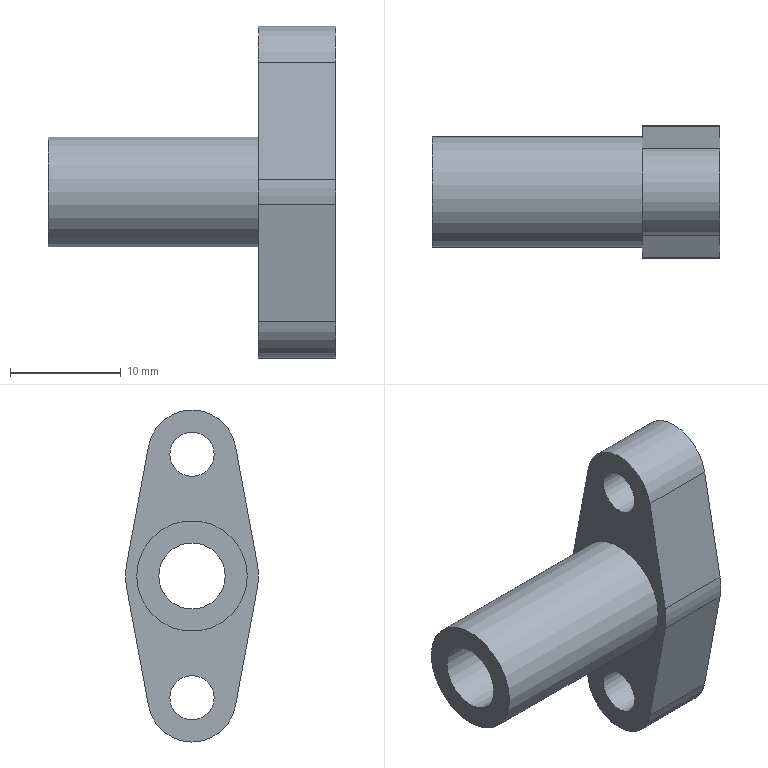Part | STEP file | 1-01.13 | 1 solid | 15 faces | box 26 x 12 x 30 mm | volume 2499 mm3 | cylinder 8 | plane 7 | commonest cylinder face diameters 4 x2 8 x2 12 x2 6 x1 10 x1
STEP:
#1=CARTESIAN_POINT('',(0.,0.,0.));
#2=DIRECTION('',(0.,0.,1.));
#3=DIRECTION('',(1.,0.,0.));
#4=AXIS2_PLACEMENT_3D('',#1,#2,#3);
#5=CARTESIAN_POINT('',(7.,5.9,-1.091));
#6=VERTEX_POINT('',#5);
#7=CARTESIAN_POINT('',(7.,5.9,1.091));
#8=VERTEX_POINT('',#7);
#9=CARTESIAN_POINT('',(7.,0.,0.));
#10=DIRECTION('',(1.,0.,0.));
#11=DIRECTION('',(0.,0.9833,-0.1818));
#12=AXIS2_PLACEMENT_3D('',#9,#10,#11);
#13=CIRCLE('',#12,6.);
#14=CARTESIAN_POINT('',(7.,8.898,0.));
#15=DIRECTION('',(1.,0.,0.));
#16=DIRECTION('',(0.,1.,0.));
#17=AXIS2_PLACEMENT_3D('',#14,#15,#16);
#18=PLANE('',#17);
#19=CARTESIAN_POINT('',(-8.898,0.));
#20=DIRECTION('',(0.9833,-0.1818));
#21=AXIS2_PLACEMENT_2D('',#19,#20);
#22=CIRCLE('',#21,6.);
#23=(GEOMETRIC_REPRESENTATION_CONTEXT(2)PARAMETRIC_REPRESENTATION_CONTEXT()REPRESENTATION_CONTEXT('',''));
#24=DEFINITIONAL_REPRESENTATION('',(#22),#23);
#25=PCURVE('',#18,#24);
#26=CARTESIAN_POINT('',(0.,0.,0.));
#27=DIRECTION('',(1.,0.,0.));
#28=DIRECTION('',(0.,0.9833,-0.1818));
#29=AXIS2_PLACEMENT_3D('',#26,#27,#28);
#30=CYLINDRICAL_SURFACE('',#29,6.);
#31=CARTESIAN_POINT('',(0.,7.));
#32=DIRECTION('',(1.,0.));
#33=VECTOR('',#32,1.);
#34=LINE('',#31,#33);
#35=(GEOMETRIC_REPRESENTATION_CONTEXT(2)PARAMETRIC_REPRESENTATION_CONTEXT()REPRESENTATION_CONTEXT('',''));
#36=DEFINITIONAL_REPRESENTATION('',(#34),#35);
#37=PCURVE('',#30,#36);
#38=SURFACE_CURVE('',#13,(#25,#37),.PCURVE_S1.);
#39=EDGE_CURVE('',#6,#8,#38,.T.);
#40=ORIENTED_EDGE('',*,*,#39,.T.);
#41=CARTESIAN_POINT('',(7.,3.933,11.727));
#42=VERTEX_POINT('',#41);
#43=CARTESIAN_POINT('',(7.,5.9,1.091));
#44=DIRECTION('',(0.,-0.1818,0.9833));
#45=VECTOR('',#44,1.);
#46=LINE('',#43,#45);
#47=CARTESIAN_POINT('',(-2.998,1.091));
#48=DIRECTION('',(-0.1818,0.9833));
#49=VECTOR('',#48,1.);
#50=LINE('',#47,#49);
#51=(GEOMETRIC_REPRESENTATION_CONTEXT(2)PARAMETRIC_REPRESENTATION_CONTEXT()REPRESENTATION_CONTEXT('',''));
#52=DEFINITIONAL_REPRESENTATION('',(#50),#51);
#53=PCURVE('',#18,#52);
#54=CARTESIAN_POINT('',(3.5,4.917,6.409));
#55=DIRECTION('',(0.,0.9833,0.1818));
#56=DIRECTION('',(0.,-0.1818,0.9833));
#57=AXIS2_PLACEMENT_3D('',#54,#55,#56);
#58=PLANE('',#57);
#59=CARTESIAN_POINT('',(-5.408,3.5));
#60=DIRECTION('',(1.,0.));
#61=VECTOR('',#60,1.);
#62=LINE('',#59,#61);
#63=(GEOMETRIC_REPRESENTATION_CONTEXT(2)PARAMETRIC_REPRESENTATION_CONTEXT()REPRESENTATION_CONTEXT('',''));
#64=DEFINITIONAL_REPRESENTATION('',(#62),#63);
#65=PCURVE('',#58,#64);
#66=SURFACE_CURVE('',#46,(#53,#65),.PCURVE_S1.);
#67=EDGE_CURVE('',#8,#42,#66,.T.);
#68=ORIENTED_EDGE('',*,*,#67,.T.);
#69=CARTESIAN_POINT('',(7.,-3.933,11.727));
#70=VERTEX_POINT('',#69);
#71=CARTESIAN_POINT('',(7.,0.,11.));
#72=DIRECTION('',(1.,0.,0.));
#73=DIRECTION('',(0.,0.9833,0.1818));
#74=AXIS2_PLACEMENT_3D('',#71,#72,#73);
#75=CIRCLE('',#74,4.);
#76=CARTESIAN_POINT('',(-8.898,11.));
#77=DIRECTION('',(0.9833,0.1818));
#78=AXIS2_PLACEMENT_2D('',#76,#77);
#79=CIRCLE('',#78,4.);
#80=(GEOMETRIC_REPRESENTATION_CONTEXT(2)PARAMETRIC_REPRESENTATION_CONTEXT()REPRESENTATION_CONTEXT('',''));
#81=DEFINITIONAL_REPRESENTATION('',(#79),#80);
#82=PCURVE('',#18,#81);
#83=CARTESIAN_POINT('',(0.,0.,11.));
#84=DIRECTION('',(1.,0.,0.));
#85=DIRECTION('',(0.,0.9833,0.1818));
#86=AXIS2_PLACEMENT_3D('',#83,#84,#85);
#87=CYLINDRICAL_SURFACE('',#86,4.);
#88=CARTESIAN_POINT('',(0.,7.));
#89=DIRECTION('',(1.,0.));
#90=VECTOR('',#89,1.);
#91=LINE('',#88,#90);
#92=(GEOMETRIC_REPRESENTATION_CONTEXT(2)PARAMETRIC_REPRESENTATION_CONTEXT()REPRESENTATION_CONTEXT('',''));
#93=DEFINITIONAL_REPRESENTATION('',(#91),#92);
#94=PCURVE('',#87,#93);
#95=SURFACE_CURVE('',#75,(#82,#94),.PCURVE_S1.);
#96=EDGE_CURVE('',#42,#70,#95,.T.);
#97=ORIENTED_EDGE('',*,*,#96,.T.);
#98=CARTESIAN_POINT('',(7.,-5.9,1.091));
#99=VERTEX_POINT('',#98);
#100=CARTESIAN_POINT('',(7.,-3.933,11.727));
#101=DIRECTION('',(0.,-0.1818,-0.9833));
#102=VECTOR('',#101,1.);
#103=LINE('',#100,#102);
#104=CARTESIAN_POINT('',(-12.832,11.727));
#105=DIRECTION('',(-0.1818,-0.9833));
#106=VECTOR('',#105,1.);
#107=LINE('',#104,#106);
#108=(GEOMETRIC_REPRESENTATION_CONTEXT(2)PARAMETRIC_REPRESENTATION_CONTEXT()REPRESENTATION_CONTEXT('',''));
#109=DEFINITIONAL_REPRESENTATION('',(#107),#108);
#110=PCURVE('',#18,#109);
#111=CARTESIAN_POINT('',(3.5,-4.917,6.409));
#112=DIRECTION('',(0.,-0.9833,0.1818));
#113=DIRECTION('',(0.,-0.1818,-0.9833));
#114=AXIS2_PLACEMENT_3D('',#111,#112,#113);
#115=PLANE('',#114);
#116=CARTESIAN_POINT('',(-5.408,3.5));
#117=DIRECTION('',(1.,0.));
#118=VECTOR('',#117,1.);
#119=LINE('',#116,#118);
#120=(GEOMETRIC_REPRESENTATION_CONTEXT(2)PARAMETRIC_REPRESENTATION_CONTEXT()REPRESENTATION_CONTEXT('',''));
#121=DEFINITIONAL_REPRESENTATION('',(#119),#120);
#122=PCURVE('',#115,#121);
#123=SURFACE_CURVE('',#103,(#110,#122),.PCURVE_S1.);
#124=EDGE_CURVE('',#70,#99,#123,.T.);
#125=ORIENTED_EDGE('',*,*,#124,.T.);
#126=CARTESIAN_POINT('',(7.,-5.9,-1.091));
#127=VERTEX_POINT('',#126);
#128=CARTESIAN_POINT('',(7.,0.,0.));
#129=DIRECTION('',(1.,0.,0.));
#130=DIRECTION('',(0.,-0.9833,0.1818));
#131=AXIS2_PLACEMENT_3D('',#128,#129,#130);
#132=CIRCLE('',#131,6.);
#133=CARTESIAN_POINT('',(-8.898,0.));
#134=DIRECTION('',(-0.9833,0.1818));
#135=AXIS2_PLACEMENT_2D('',#133,#134);
#136=CIRCLE('',#135,6.);
#137=(GEOMETRIC_REPRESENTATION_CONTEXT(2)PARAMETRIC_REPRESENTATION_CONTEXT()REPRESENTATION_CONTEXT('',''));
#138=DEFINITIONAL_REPRESENTATION('',(#136),#137);
#139=PCURVE('',#18,#138);
#140=CARTESIAN_POINT('',(0.,0.,0.));
#141=DIRECTION('',(1.,0.,0.));
#142=DIRECTION('',(0.,-0.9833,0.1818));
#143=AXIS2_PLACEMENT_3D('',#140,#141,#142);
#144=CYLINDRICAL_SURFACE('',#143,6.);
#145=CARTESIAN_POINT('',(0.,7.));
#146=DIRECTION('',(1.,0.));
#147=VECTOR('',#146,1.);
#148=LINE('',#145,#147);
#149=(GEOMETRIC_REPRESENTATION_CONTEXT(2)PARAMETRIC_REPRESENTATION_CONTEXT()REPRESENTATION_CONTEXT('',''));
#150=DEFINITIONAL_REPRESENTATION('',(#148),#149);
#151=PCURVE('',#144,#150);
#152=SURFACE_CURVE('',#132,(#139,#151),.PCURVE_S1.);
#153=EDGE_CURVE('',#99,#127,#152,.T.);
#154=ORIENTED_EDGE('',*,*,#153,.T.);
#155=CARTESIAN_POINT('',(7.,-3.933,-11.727));
#156=VERTEX_POINT('',#155);
#157=CARTESIAN_POINT('',(7.,-5.9,-1.091));
#158=DIRECTION('',(0.,0.1818,-0.9833));
#159=VECTOR('',#158,1.);
#160=LINE('',#157,#159);
#161=CARTESIAN_POINT('',(-14.798,-1.091));
#162=DIRECTION('',(0.1818,-0.9833));
#163=VECTOR('',#162,1.);
#164=LINE('',#161,#163);
#165=(GEOMETRIC_REPRESENTATION_CONTEXT(2)PARAMETRIC_REPRESENTATION_CONTEXT()REPRESENTATION_CONTEXT('',''));
#166=DEFINITIONAL_REPRESENTATION('',(#164),#165);
#167=PCURVE('',#18,#166);
#168=CARTESIAN_POINT('',(3.5,-4.917,-6.409));
#169=DIRECTION('',(0.,-0.9833,-0.1818));
#170=DIRECTION('',(0.,0.1818,-0.9833));
#171=AXIS2_PLACEMENT_3D('',#168,#169,#170);
#172=PLANE('',#171);
#173=CARTESIAN_POINT('',(-5.408,3.5));
#174=DIRECTION('',(1.,0.));
#175=VECTOR('',#174,1.);
#176=LINE('',#173,#175);
#177=(GEOMETRIC_REPRESENTATION_CONTEXT(2)PARAMETRIC_REPRESENTATION_CONTEXT()REPRESENTATION_CONTEXT('',''));
#178=DEFINITIONAL_REPRESENTATION('',(#176),#177);
#179=PCURVE('',#172,#178);
#180=SURFACE_CURVE('',#160,(#167,#179),.PCURVE_S1.);
#181=EDGE_CURVE('',#127,#156,#180,.T.);
#182=ORIENTED_EDGE('',*,*,#181,.T.);
#183=CARTESIAN_POINT('',(7.,3.933,-11.727));
#184=VERTEX_POINT('',#183);
#185=CARTESIAN_POINT('',(7.,0.,-11.));
#186=DIRECTION('',(1.,0.,0.));
#187=DIRECTION('',(0.,-0.9833,-0.1818));
#188=AXIS2_PLACEMENT_3D('',#185,#186,#187);
#189=CIRCLE('',#188,4.);
#190=CARTESIAN_POINT('',(-8.898,-11.));
#191=DIRECTION('',(-0.9833,-0.1818));
#192=AXIS2_PLACEMENT_2D('',#190,#191);
#193=CIRCLE('',#192,4.);
#194=(GEOMETRIC_REPRESENTATION_CONTEXT(2)PARAMETRIC_REPRESENTATION_CONTEXT()REPRESENTATION_CONTEXT('',''));
#195=DEFINITIONAL_REPRESENTATION('',(#193),#194);
#196=PCURVE('',#18,#195);
#197=CARTESIAN_POINT('',(0.,0.,-11.));
#198=DIRECTION('',(1.,0.,0.));
#199=DIRECTION('',(0.,-0.9833,-0.1818));
#200=AXIS2_PLACEMENT_3D('',#197,#198,#199);
#201=CYLINDRICAL_SURFACE('',#200,4.);
#202=CARTESIAN_POINT('',(0.,7.));
#203=DIRECTION('',(1.,0.));
#204=VECTOR('',#203,1.);
#205=LINE('',#202,#204);
#206=(GEOMETRIC_REPRESENTATION_CONTEXT(2)PARAMETRIC_REPRESENTATION_CONTEXT()REPRESENTATION_CONTEXT('',''));
#207=DEFINITIONAL_REPRESENTATION('',(#205),#206);
#208=PCURVE('',#201,#207);
#209=SURFACE_CURVE('',#189,(#196,#208),.PCURVE_S1.);
#210=EDGE_CURVE('',#156,#184,#209,.T.);
#211=ORIENTED_EDGE('',*,*,#210,.T.);
#212=CARTESIAN_POINT('',(7.,3.933,-11.727));
#213=DIRECTION('',(0.,0.1818,0.9833));
#214=VECTOR('',#213,1.);
#215=LINE('',#212,#214);
#216=CARTESIAN_POINT('',(-4.965,-11.727));
#217=DIRECTION('',(0.1818,0.9833));
#218=VECTOR('',#217,1.);
#219=LINE('',#216,#218);
#220=(GEOMETRIC_REPRESENTATION_CONTEXT(2)PARAMETRIC_REPRESENTATION_CONTEXT()REPRESENTATION_CONTEXT('',''));
#221=DEFINITIONAL_REPRESENTATION('',(#219),#220);
#222=PCURVE('',#18,#221);
#223=CARTESIAN_POINT('',(3.5,4.917,-6.409));
#224=DIRECTION('',(0.,0.9833,-0.1818));
#225=DIRECTION('',(0.,0.1818,0.9833));
#226=AXIS2_PLACEMENT_3D('',#223,#224,#225);
#227=PLANE('',#226);
#228=CARTESIAN_POINT('',(-5.408,3.5));
#229=DIRECTION('',(1.,0.));
#230=VECTOR('',#229,1.);
#231=LINE('',#228,#230);
#232=(GEOMETRIC_REPRESENTATION_CONTEXT(2)PARAMETRIC_REPRESENTATION_CONTEXT()REPRESENTATION_CONTEXT('',''));
#233=DEFINITIONAL_REPRESENTATION('',(#231),#232);
#234=PCURVE('',#227,#233);
#235=SURFACE_CURVE('',#215,(#222,#234),.PCURVE_S1.);
#236=EDGE_CURVE('',#184,#6,#235,.T.);
#237=ORIENTED_EDGE('',*,*,#236,.T.);
#238=EDGE_LOOP('',(#40,#68,#97,#125,#154,#182,#211,#237));
#239=FACE_BOUND('',#238,.T.);
#240=CARTESIAN_POINT('',(7.,3.,0.));
#241=VERTEX_POINT('',#240);
#242=CARTESIAN_POINT('',(7.,0.,0.));
#243=DIRECTION('',(-1.,0.,0.));
#244=DIRECTION('',(0.,1.,0.));
#245=AXIS2_PLACEMENT_3D('',#242,#243,#244);
#246=CIRCLE('',#245,3.);
#247=CARTESIAN_POINT('',(-5.898,0.));
#248=CARTESIAN_POINT('',(-5.898,-5.196));
#249=CARTESIAN_POINT('',(-10.398,-2.598));
#250=CARTESIAN_POINT('',(-14.898,0.));
#251=CARTESIAN_POINT('',(-10.398,2.598));
#252=CARTESIAN_POINT('',(-5.898,5.196));
#253=CARTESIAN_POINT('',(-5.898,0.));
#254=(BOUNDED_CURVE()B_SPLINE_CURVE(2,(#247,#248,#249,#250,#251,#252,#253),.UNSPECIFIED.,.T.,.F.)B_SPLINE_CURVE_WITH_KNOTS((1,2,2,2,2,1),(-2.094,0.,2.094,4.189,6.283,8.378),.UNSPECIFIED.)CURVE()GEOMETRIC_REPRESENTATION_ITEM()RATIONAL_B_SPLINE_CURVE((1.,0.5,1.,0.5,1.,0.5,1.))REPRESENTATION_ITEM(''));
#255=(GEOMETRIC_REPRESENTATION_CONTEXT(2)PARAMETRIC_REPRESENTATION_CONTEXT()REPRESENTATION_CONTEXT('',''));
#256=DEFINITIONAL_REPRESENTATION('',(#254),#255);
#257=PCURVE('',#18,#256);
#258=CARTESIAN_POINT('',(-19.,0.,0.));
#259=DIRECTION('',(1.,0.,0.));
#260=DIRECTION('',(0.,1.,0.));
#261=AXIS2_PLACEMENT_3D('',#258,#259,#260);
#262=CYLINDRICAL_SURFACE('',#261,3.);
#263=CARTESIAN_POINT('',(6.283,26.));
#264=DIRECTION('',(-1.,0.));
#265=VECTOR('',#264,1.);
#266=LINE('',#263,#265);
#267=(GEOMETRIC_REPRESENTATION_CONTEXT(2)PARAMETRIC_REPRESENTATION_CONTEXT()REPRESENTATION_CONTEXT('',''));
#268=DEFINITIONAL_REPRESENTATION('',(#266),#267);
#269=PCURVE('',#262,#268);
#270=SURFACE_CURVE('',#246,(#257,#269),.PCURVE_S1.);
#271=EDGE_CURVE('',#241,#241,#270,.T.);
#272=ORIENTED_EDGE('',*,*,#271,.T.);
#273=EDGE_LOOP('',(#272));
#274=FACE_BOUND('',#273,.T.);
#275=CARTESIAN_POINT('',(7.,2.,11.));
#276=VERTEX_POINT('',#275);
#277=CARTESIAN_POINT('',(7.,0.,11.));
#278=DIRECTION('',(-1.,0.,0.));
#279=DIRECTION('',(0.,1.,0.));
#280=AXIS2_PLACEMENT_3D('',#277,#278,#279);
#281=CIRCLE('',#280,2.);
#282=CARTESIAN_POINT('',(-6.898,11.));
#283=CARTESIAN_POINT('',(-6.898,7.536));
#284=CARTESIAN_POINT('',(-9.898,9.268));
#285=CARTESIAN_POINT('',(-12.898,11.));
#286=CARTESIAN_POINT('',(-9.898,12.732));
#287=CARTESIAN_POINT('',(-6.898,14.464));
#288=CARTESIAN_POINT('',(-6.898,11.));
#289=(BOUNDED_CURVE()B_SPLINE_CURVE(2,(#282,#283,#284,#285,#286,#287,#288),.UNSPECIFIED.,.T.,.F.)B_SPLINE_CURVE_WITH_KNOTS((1,2,2,2,2,1),(-2.094,0.,2.094,4.189,6.283,8.378),.UNSPECIFIED.)CURVE()GEOMETRIC_REPRESENTATION_ITEM()RATIONAL_B_SPLINE_CURVE((1.,0.5,1.,0.5,1.,0.5,1.))REPRESENTATION_ITEM(''));
#290=(GEOMETRIC_REPRESENTATION_CONTEXT(2)PARAMETRIC_REPRESENTATION_CONTEXT()REPRESENTATION_CONTEXT('',''));
#291=DEFINITIONAL_REPRESENTATION('',(#289),#290);
#292=PCURVE('',#18,#291);
#293=CARTESIAN_POINT('',(0.,0.,11.));
#294=DIRECTION('',(1.,0.,0.));
#295=DIRECTION('',(0.,1.,0.));
#296=AXIS2_PLACEMENT_3D('',#293,#294,#295);
#297=CYLINDRICAL_SURFACE('',#296,2.);
#298=CARTESIAN_POINT('',(6.283,7.));
#299=DIRECTION('',(-1.,0.));
#300=VECTOR('',#299,1.);
#301=LINE('',#298,#300);
#302=(GEOMETRIC_REPRESENTATION_CONTEXT(2)PARAMETRIC_REPRESENTATION_CONTEXT()REPRESENTATION_CONTEXT('',''));
#303=DEFINITIONAL_REPRESENTATION('',(#301),#302);
#304=PCURVE('',#297,#303);
#305=SURFACE_CURVE('',#281,(#292,#304),.PCURVE_S1.);
#306=EDGE_CURVE('',#276,#276,#305,.T.);
#307=ORIENTED_EDGE('',*,*,#306,.T.);
#308=EDGE_LOOP('',(#307));
#309=FACE_BOUND('',#308,.T.);
#310=CARTESIAN_POINT('',(7.,2.,-11.));
#311=VERTEX_POINT('',#310);
#312=CARTESIAN_POINT('',(7.,0.,-11.));
#313=DIRECTION('',(-1.,0.,0.));
#314=DIRECTION('',(0.,1.,0.));
#315=AXIS2_PLACEMENT_3D('',#312,#313,#314);
#316=CIRCLE('',#315,2.);
#317=CARTESIAN_POINT('',(-6.898,-11.));
#318=CARTESIAN_POINT('',(-6.898,-14.464));
#319=CARTESIAN_POINT('',(-9.898,-12.732));
#320=CARTESIAN_POINT('',(-12.898,-11.));
#321=CARTESIAN_POINT('',(-9.898,-9.268));
#322=CARTESIAN_POINT('',(-6.898,-7.536));
#323=CARTESIAN_POINT('',(-6.898,-11.));
#324=(BOUNDED_CURVE()B_SPLINE_CURVE(2,(#317,#318,#319,#320,#321,#322,#323),.UNSPECIFIED.,.T.,.F.)B_SPLINE_CURVE_WITH_KNOTS((1,2,2,2,2,1),(-2.094,0.,2.094,4.189,6.283,8.378),.UNSPECIFIED.)CURVE()GEOMETRIC_REPRESENTATION_ITEM()RATIONAL_B_SPLINE_CURVE((1.,0.5,1.,0.5,1.,0.5,1.))REPRESENTATION_ITEM(''));
#325=(GEOMETRIC_REPRESENTATION_CONTEXT(2)PARAMETRIC_REPRESENTATION_CONTEXT()REPRESENTATION_CONTEXT('',''));
#326=DEFINITIONAL_REPRESENTATION('',(#324),#325);
#327=PCURVE('',#18,#326);
#328=CARTESIAN_POINT('',(0.,0.,-11.));
#329=DIRECTION('',(1.,0.,0.));
#330=DIRECTION('',(0.,1.,0.));
#331=AXIS2_PLACEMENT_3D('',#328,#329,#330);
#332=CYLINDRICAL_SURFACE('',#331,2.);
#333=CARTESIAN_POINT('',(6.283,7.));
#334=DIRECTION('',(-1.,0.));
#335=VECTOR('',#334,1.);
#336=LINE('',#333,#335);
#337=(GEOMETRIC_REPRESENTATION_CONTEXT(2)PARAMETRIC_REPRESENTATION_CONTEXT()REPRESENTATION_CONTEXT('',''));
#338=DEFINITIONAL_REPRESENTATION('',(#336),#337);
#339=PCURVE('',#332,#338);
#340=SURFACE_CURVE('',#316,(#327,#339),.PCURVE_S1.);
#341=EDGE_CURVE('',#311,#311,#340,.T.);
#342=ORIENTED_EDGE('',*,*,#341,.T.);
#343=EDGE_LOOP('',(#342));
#344=FACE_BOUND('',#343,.T.);
#345=ADVANCED_FACE('',(#239,#274,#309,#344),#18,.T.);
#346=CARTESIAN_POINT('',(0.,5.9,-1.091));
#347=VERTEX_POINT('',#346);
#348=CARTESIAN_POINT('',(0.,5.9,1.091));
#349=VERTEX_POINT('',#348);
#350=CARTESIAN_POINT('',(0.,0.,0.));
#351=DIRECTION('',(1.,0.,0.));
#352=DIRECTION('',(0.,0.9833,-0.1818));
#353=AXIS2_PLACEMENT_3D('',#350,#351,#352);
#354=CIRCLE('',#353,6.);
#355=CARTESIAN_POINT('',(0.,0.));
#356=DIRECTION('',(1.,0.));
#357=VECTOR('',#356,1.);
#358=LINE('',#355,#357);
#359=(GEOMETRIC_REPRESENTATION_CONTEXT(2)PARAMETRIC_REPRESENTATION_CONTEXT()REPRESENTATION_CONTEXT('',''));
#360=DEFINITIONAL_REPRESENTATION('',(#358),#359);
#361=PCURVE('',#30,#360);
#362=CARTESIAN_POINT('',(0.,8.898,0.));
#363=DIRECTION('',(1.,0.,0.));
#364=DIRECTION('',(0.,1.,0.));
#365=AXIS2_PLACEMENT_3D('',#362,#363,#364);
#366=PLANE('',#365);
#367=CARTESIAN_POINT('',(-8.898,0.));
#368=DIRECTION('',(0.9833,-0.1818));
#369=AXIS2_PLACEMENT_2D('',#367,#368);
#370=CIRCLE('',#369,6.);
#371=(GEOMETRIC_REPRESENTATION_CONTEXT(2)PARAMETRIC_REPRESENTATION_CONTEXT()REPRESENTATION_CONTEXT('',''));
#372=DEFINITIONAL_REPRESENTATION('',(#370),#371);
#373=PCURVE('',#366,#372);
#374=SURFACE_CURVE('',#354,(#361,#373),.PCURVE_S1.);
#375=EDGE_CURVE('',#347,#349,#374,.T.);
#376=ORIENTED_EDGE('',*,*,#375,.T.);
#377=CARTESIAN_POINT('',(0.,5.9,1.091));
#378=DIRECTION('',(1.,0.,0.));
#379=VECTOR('',#378,1.);
#380=LINE('',#377,#379);
#381=CARTESIAN_POINT('',(0.3657,0.));
#382=DIRECTION('',(0.,1.));
#383=VECTOR('',#382,1.);
#384=LINE('',#381,#383);
#385=(GEOMETRIC_REPRESENTATION_CONTEXT(2)PARAMETRIC_REPRESENTATION_CONTEXT()REPRESENTATION_CONTEXT('',''));
#386=DEFINITIONAL_REPRESENTATION('',(#384),#385);
#387=PCURVE('',#30,#386);
#388=CARTESIAN_POINT('',(-5.408,-3.5));
#389=DIRECTION('',(0.,1.));
#390=VECTOR('',#389,1.);
#391=LINE('',#388,#390);
#392=(GEOMETRIC_REPRESENTATION_CONTEXT(2)PARAMETRIC_REPRESENTATION_CONTEXT()REPRESENTATION_CONTEXT('',''));
#393=DEFINITIONAL_REPRESENTATION('',(#391),#392);
#394=PCURVE('',#58,#393);
#395=SURFACE_CURVE('',#380,(#387,#394),.PCURVE_S1.);
#396=EDGE_CURVE('',#349,#8,#395,.T.);
#397=ORIENTED_EDGE('',*,*,#396,.T.);
#398=ORIENTED_EDGE('',*,*,#39,.F.);
#399=CARTESIAN_POINT('',(0.,5.9,-1.091));
#400=DIRECTION('',(1.,0.,0.));
#401=VECTOR('',#400,1.);
#402=LINE('',#399,#401);
#403=CARTESIAN_POINT('',(0.,0.));
#404=DIRECTION('',(0.,1.));
#405=VECTOR('',#404,1.);
#406=LINE('',#403,#405);
#407=(GEOMETRIC_REPRESENTATION_CONTEXT(2)PARAMETRIC_REPRESENTATION_CONTEXT()REPRESENTATION_CONTEXT('',''));
#408=DEFINITIONAL_REPRESENTATION('',(#406),#407);
#409=PCURVE('',#30,#408);
#410=CARTESIAN_POINT('',(5.408,-3.5));
#411=DIRECTION('',(0.,1.));
#412=VECTOR('',#411,1.);
#413=LINE('',#410,#412);
#414=(GEOMETRIC_REPRESENTATION_CONTEXT(2)PARAMETRIC_REPRESENTATION_CONTEXT()REPRESENTATION_CONTEXT('',''));
#415=DEFINITIONAL_REPRESENTATION('',(#413),#414);
#416=PCURVE('',#227,#415);
#417=SURFACE_CURVE('',#402,(#409,#416),.PCURVE_S1.);
#418=EDGE_CURVE('',#347,#6,#417,.T.);
#419=ORIENTED_EDGE('',*,*,#418,.F.);
#420=EDGE_LOOP('',(#376,#397,#398,#419));
#421=FACE_BOUND('',#420,.T.);
#422=ADVANCED_FACE('',(#421),#30,.T.);
#423=CARTESIAN_POINT('',(0.,3.933,11.727));
#424=VERTEX_POINT('',#423);
#425=CARTESIAN_POINT('',(0.,5.9,1.091));
#426=DIRECTION('',(0.,-0.1818,0.9833));
#427=VECTOR('',#426,1.);
#428=LINE('',#425,#427);
#429=CARTESIAN_POINT('',(-5.408,-3.5));
#430=DIRECTION('',(1.,0.));
#431=VECTOR('',#430,1.);
#432=LINE('',#429,#431);
#433=(GEOMETRIC_REPRESENTATION_CONTEXT(2)PARAMETRIC_REPRESENTATION_CONTEXT()REPRESENTATION_CONTEXT('',''));
#434=DEFINITIONAL_REPRESENTATION('',(#432),#433);
#435=PCURVE('',#58,#434);
#436=CARTESIAN_POINT('',(-2.998,1.091));
#437=DIRECTION('',(-0.1818,0.9833));
#438=VECTOR('',#437,1.);
#439=LINE('',#436,#438);
#440=(GEOMETRIC_REPRESENTATION_CONTEXT(2)PARAMETRIC_REPRESENTATION_CONTEXT()REPRESENTATION_CONTEXT('',''));
#441=DEFINITIONAL_REPRESENTATION('',(#439),#440);
#442=PCURVE('',#366,#441);
#443=SURFACE_CURVE('',#428,(#435,#442),.PCURVE_S1.);
#444=EDGE_CURVE('',#349,#424,#443,.T.);
#445=ORIENTED_EDGE('',*,*,#444,.T.);
#446=CARTESIAN_POINT('',(0.,3.933,11.727));
#447=DIRECTION('',(1.,0.,0.));
#448=VECTOR('',#447,1.);
#449=LINE('',#446,#448);
#450=CARTESIAN_POINT('',(5.408,-3.5));
#451=DIRECTION('',(0.,1.));
#452=VECTOR('',#451,1.);
#453=LINE('',#450,#452);
#454=(GEOMETRIC_REPRESENTATION_CONTEXT(2)PARAMETRIC_REPRESENTATION_CONTEXT()REPRESENTATION_CONTEXT('',''));
#455=DEFINITIONAL_REPRESENTATION('',(#453),#454);
#456=PCURVE('',#58,#455);
#457=CARTESIAN_POINT('',(0.,0.));
#458=DIRECTION('',(0.,1.));
#459=VECTOR('',#458,1.);
#460=LINE('',#457,#459);
#461=(GEOMETRIC_REPRESENTATION_CONTEXT(2)PARAMETRIC_REPRESENTATION_CONTEXT()REPRESENTATION_CONTEXT('',''));
#462=DEFINITIONAL_REPRESENTATION('',(#460),#461);
#463=PCURVE('',#87,#462);
#464=SURFACE_CURVE('',#449,(#456,#463),.PCURVE_S1.);
#465=EDGE_CURVE('',#424,#42,#464,.T.);
#466=ORIENTED_EDGE('',*,*,#465,.T.);
#467=ORIENTED_EDGE('',*,*,#67,.F.);
#468=ORIENTED_EDGE('',*,*,#396,.F.);
#469=EDGE_LOOP('',(#445,#466,#467,#468));
#470=FACE_BOUND('',#469,.T.);
#471=ADVANCED_FACE('',(#470),#58,.T.);
#472=CARTESIAN_POINT('',(0.,-3.933,11.727));
#473=VERTEX_POINT('',#472);
#474=CARTESIAN_POINT('',(0.,0.,11.));
#475=DIRECTION('',(1.,0.,0.));
#476=DIRECTION('',(0.,0.9833,0.1818));
#477=AXIS2_PLACEMENT_3D('',#474,#475,#476);
#478=CIRCLE('',#477,4.);
#479=CARTESIAN_POINT('',(0.,0.));
#480=DIRECTION('',(1.,0.));
#481=VECTOR('',#480,1.);
#482=LINE('',#479,#481);
#483=(GEOMETRIC_REPRESENTATION_CONTEXT(2)PARAMETRIC_REPRESENTATION_CONTEXT()REPRESENTATION_CONTEXT('',''));
#484=DEFINITIONAL_REPRESENTATION('',(#482),#483);
#485=PCURVE('',#87,#484);
#486=CARTESIAN_POINT('',(-8.898,11.));
#487=DIRECTION('',(0.9833,0.1818));
#488=AXIS2_PLACEMENT_2D('',#486,#487);
#489=CIRCLE('',#488,4.);
#490=(GEOMETRIC_REPRESENTATION_CONTEXT(2)PARAMETRIC_REPRESENTATION_CONTEXT()REPRESENTATION_CONTEXT('',''));
#491=DEFINITIONAL_REPRESENTATION('',(#489),#490);
#492=PCURVE('',#366,#491);
#493=SURFACE_CURVE('',#478,(#485,#492),.PCURVE_S1.);
#494=EDGE_CURVE('',#424,#473,#493,.T.);
#495=ORIENTED_EDGE('',*,*,#494,.T.);
#496=CARTESIAN_POINT('',(0.,-3.933,11.727));
#497=DIRECTION('',(1.,0.,0.));
#498=VECTOR('',#497,1.);
#499=LINE('',#496,#498);
#500=CARTESIAN_POINT('',(2.776,0.));
#501=DIRECTION('',(0.,1.));
#502=VECTOR('',#501,1.);
#503=LINE('',#500,#502);
#504=(GEOMETRIC_REPRESENTATION_CONTEXT(2)PARAMETRIC_REPRESENTATION_CONTEXT()REPRESENTATION_CONTEXT('',''));
#505=DEFINITIONAL_REPRESENTATION('',(#503),#504);
#506=PCURVE('',#87,#505);
#507=CARTESIAN_POINT('',(-5.408,-3.5));
#508=DIRECTION('',(0.,1.));
#509=VECTOR('',#508,1.);
#510=LINE('',#507,#509);
#511=(GEOMETRIC_REPRESENTATION_CONTEXT(2)PARAMETRIC_REPRESENTATION_CONTEXT()REPRESENTATION_CONTEXT('',''));
#512=DEFINITIONAL_REPRESENTATION('',(#510),#511);
#513=PCURVE('',#115,#512);
#514=SURFACE_CURVE('',#499,(#506,#513),.PCURVE_S1.);
#515=EDGE_CURVE('',#473,#70,#514,.T.);
#516=ORIENTED_EDGE('',*,*,#515,.T.);
#517=ORIENTED_EDGE('',*,*,#96,.F.);
#518=ORIENTED_EDGE('',*,*,#465,.F.);
#519=EDGE_LOOP('',(#495,#516,#517,#518));
#520=FACE_BOUND('',#519,.T.);
#521=ADVANCED_FACE('',(#520),#87,.T.);
#522=CARTESIAN_POINT('',(0.,-5.9,1.091));
#523=VERTEX_POINT('',#522);
#524=CARTESIAN_POINT('',(0.,-3.933,11.727));
#525=DIRECTION('',(0.,-0.1818,-0.9833));
#526=VECTOR('',#525,1.);
#527=LINE('',#524,#526);
#528=CARTESIAN_POINT('',(-5.408,-3.5));
#529=DIRECTION('',(1.,0.));
#530=VECTOR('',#529,1.);
#531=LINE('',#528,#530);
#532=(GEOMETRIC_REPRESENTATION_CONTEXT(2)PARAMETRIC_REPRESENTATION_CONTEXT()REPRESENTATION_CONTEXT('',''));
#533=DEFINITIONAL_REPRESENTATION('',(#531),#532);
#534=PCURVE('',#115,#533);
#535=CARTESIAN_POINT('',(-12.832,11.727));
#536=DIRECTION('',(-0.1818,-0.9833));
#537=VECTOR('',#536,1.);
#538=LINE('',#535,#537);
#539=(GEOMETRIC_REPRESENTATION_CONTEXT(2)PARAMETRIC_REPRESENTATION_CONTEXT()REPRESENTATION_CONTEXT('',''));
#540=DEFINITIONAL_REPRESENTATION('',(#538),#539);
#541=PCURVE('',#366,#540);
#542=SURFACE_CURVE('',#527,(#534,#541),.PCURVE_S1.);
#543=EDGE_CURVE('',#473,#523,#542,.T.);
#544=ORIENTED_EDGE('',*,*,#543,.T.);
#545=CARTESIAN_POINT('',(0.,-5.9,1.091));
#546=DIRECTION('',(1.,0.,0.));
#547=VECTOR('',#546,1.);
#548=LINE('',#545,#547);
#549=CARTESIAN_POINT('',(5.408,-3.5));
#550=DIRECTION('',(0.,1.));
#551=VECTOR('',#550,1.);
#552=LINE('',#549,#551);
#553=(GEOMETRIC_REPRESENTATION_CONTEXT(2)PARAMETRIC_REPRESENTATION_CONTEXT()REPRESENTATION_CONTEXT('',''));
#554=DEFINITIONAL_REPRESENTATION('',(#552),#553);
#555=PCURVE('',#115,#554);
#556=CARTESIAN_POINT('',(0.,0.));
#557=DIRECTION('',(0.,1.));
#558=VECTOR('',#557,1.);
#559=LINE('',#556,#558);
#560=(GEOMETRIC_REPRESENTATION_CONTEXT(2)PARAMETRIC_REPRESENTATION_CONTEXT()REPRESENTATION_CONTEXT('',''));
#561=DEFINITIONAL_REPRESENTATION('',(#559),#560);
#562=PCURVE('',#144,#561);
#563=SURFACE_CURVE('',#548,(#555,#562),.PCURVE_S1.);
#564=EDGE_CURVE('',#523,#99,#563,.T.);
#565=ORIENTED_EDGE('',*,*,#564,.T.);
#566=ORIENTED_EDGE('',*,*,#124,.F.);
#567=ORIENTED_EDGE('',*,*,#515,.F.);
#568=EDGE_LOOP('',(#544,#565,#566,#567));
#569=FACE_BOUND('',#568,.T.);
#570=ADVANCED_FACE('',(#569),#115,.T.);
#571=CARTESIAN_POINT('',(0.,-5.9,-1.091));
#572=VERTEX_POINT('',#571);
#573=CARTESIAN_POINT('',(0.,0.,0.));
#574=DIRECTION('',(1.,0.,0.));
#575=DIRECTION('',(0.,-0.9833,0.1818));
#576=AXIS2_PLACEMENT_3D('',#573,#574,#575);
#577=CIRCLE('',#576,6.);
#578=CARTESIAN_POINT('',(0.,0.));
#579=DIRECTION('',(1.,0.));
#580=VECTOR('',#579,1.);
#581=LINE('',#578,#580);
#582=(GEOMETRIC_REPRESENTATION_CONTEXT(2)PARAMETRIC_REPRESENTATION_CONTEXT()REPRESENTATION_CONTEXT('',''));
#583=DEFINITIONAL_REPRESENTATION('',(#581),#582);
#584=PCURVE('',#144,#583);
#585=CARTESIAN_POINT('',(-8.898,0.));
#586=DIRECTION('',(-0.9833,0.1818));
#587=AXIS2_PLACEMENT_2D('',#585,#586);
#588=CIRCLE('',#587,6.);
#589=(GEOMETRIC_REPRESENTATION_CONTEXT(2)PARAMETRIC_REPRESENTATION_CONTEXT()REPRESENTATION_CONTEXT('',''));
#590=DEFINITIONAL_REPRESENTATION('',(#588),#589);
#591=PCURVE('',#366,#590);
#592=SURFACE_CURVE('',#577,(#584,#591),.PCURVE_S1.);
#593=EDGE_CURVE('',#523,#572,#592,.T.);
#594=ORIENTED_EDGE('',*,*,#593,.T.);
#595=CARTESIAN_POINT('',(0.,-5.9,-1.091));
#596=DIRECTION('',(1.,0.,0.));
#597=VECTOR('',#596,1.);
#598=LINE('',#595,#597);
#599=CARTESIAN_POINT('',(0.3657,0.));
#600=DIRECTION('',(0.,1.));
#601=VECTOR('',#600,1.);
#602=LINE('',#599,#601);
#603=(GEOMETRIC_REPRESENTATION_CONTEXT(2)PARAMETRIC_REPRESENTATION_CONTEXT()REPRESENTATION_CONTEXT('',''));
#604=DEFINITIONAL_REPRESENTATION('',(#602),#603);
#605=PCURVE('',#144,#604);
#606=CARTESIAN_POINT('',(-5.408,-3.5));
#607=DIRECTION('',(0.,1.));
#608=VECTOR('',#607,1.);
#609=LINE('',#606,#608);
#610=(GEOMETRIC_REPRESENTATION_CONTEXT(2)PARAMETRIC_REPRESENTATION_CONTEXT()REPRESENTATION_CONTEXT('',''));
#611=DEFINITIONAL_REPRESENTATION('',(#609),#610);
#612=PCURVE('',#172,#611);
#613=SURFACE_CURVE('',#598,(#605,#612),.PCURVE_S1.);
#614=EDGE_CURVE('',#572,#127,#613,.T.);
#615=ORIENTED_EDGE('',*,*,#614,.T.);
#616=ORIENTED_EDGE('',*,*,#153,.F.);
#617=ORIENTED_EDGE('',*,*,#564,.F.);
#618=EDGE_LOOP('',(#594,#615,#616,#617));
#619=FACE_BOUND('',#618,.T.);
#620=ADVANCED_FACE('',(#619),#144,.T.);
#621=CARTESIAN_POINT('',(0.,-3.933,-11.727));
#622=VERTEX_POINT('',#621);
#623=CARTESIAN_POINT('',(0.,-5.9,-1.091));
#624=DIRECTION('',(0.,0.1818,-0.9833));
#625=VECTOR('',#624,1.);
#626=LINE('',#623,#625);
#627=CARTESIAN_POINT('',(-5.408,-3.5));
#628=DIRECTION('',(1.,0.));
#629=VECTOR('',#628,1.);
#630=LINE('',#627,#629);
#631=(GEOMETRIC_REPRESENTATION_CONTEXT(2)PARAMETRIC_REPRESENTATION_CONTEXT()REPRESENTATION_CONTEXT('',''));
#632=DEFINITIONAL_REPRESENTATION('',(#630),#631);
#633=PCURVE('',#172,#632);
#634=CARTESIAN_POINT('',(-14.798,-1.091));
#635=DIRECTION('',(0.1818,-0.9833));
#636=VECTOR('',#635,1.);
#637=LINE('',#634,#636);
#638=(GEOMETRIC_REPRESENTATION_CONTEXT(2)PARAMETRIC_REPRESENTATION_CONTEXT()REPRESENTATION_CONTEXT('',''));
#639=DEFINITIONAL_REPRESENTATION('',(#637),#638);
#640=PCURVE('',#366,#639);
#641=SURFACE_CURVE('',#626,(#633,#640),.PCURVE_S1.);
#642=EDGE_CURVE('',#572,#622,#641,.T.);
#643=ORIENTED_EDGE('',*,*,#642,.T.);
#644=CARTESIAN_POINT('',(0.,-3.933,-11.727));
#645=DIRECTION('',(1.,0.,0.));
#646=VECTOR('',#645,1.);
#647=LINE('',#644,#646);
#648=CARTESIAN_POINT('',(5.408,-3.5));
#649=DIRECTION('',(0.,1.));
#650=VECTOR('',#649,1.);
#651=LINE('',#648,#650);
#652=(GEOMETRIC_REPRESENTATION_CONTEXT(2)PARAMETRIC_REPRESENTATION_CONTEXT()REPRESENTATION_CONTEXT('',''));
#653=DEFINITIONAL_REPRESENTATION('',(#651),#652);
#654=PCURVE('',#172,#653);
#655=CARTESIAN_POINT('',(0.,0.));
#656=DIRECTION('',(0.,1.));
#657=VECTOR('',#656,1.);
#658=LINE('',#655,#657);
#659=(GEOMETRIC_REPRESENTATION_CONTEXT(2)PARAMETRIC_REPRESENTATION_CONTEXT()REPRESENTATION_CONTEXT('',''));
#660=DEFINITIONAL_REPRESENTATION('',(#658),#659);
#661=PCURVE('',#201,#660);
#662=SURFACE_CURVE('',#647,(#654,#661),.PCURVE_S1.);
#663=EDGE_CURVE('',#622,#156,#662,.T.);
#664=ORIENTED_EDGE('',*,*,#663,.T.);
#665=ORIENTED_EDGE('',*,*,#181,.F.);
#666=ORIENTED_EDGE('',*,*,#614,.F.);
#667=EDGE_LOOP('',(#643,#664,#665,#666));
#668=FACE_BOUND('',#667,.T.);
#669=ADVANCED_FACE('',(#668),#172,.T.);
#670=CARTESIAN_POINT('',(0.,3.933,-11.727));
#671=VERTEX_POINT('',#670);
#672=CARTESIAN_POINT('',(0.,0.,-11.));
#673=DIRECTION('',(1.,0.,0.));
#674=DIRECTION('',(0.,-0.9833,-0.1818));
#675=AXIS2_PLACEMENT_3D('',#672,#673,#674);
#676=CIRCLE('',#675,4.);
#677=CARTESIAN_POINT('',(0.,0.));
#678=DIRECTION('',(1.,0.));
#679=VECTOR('',#678,1.);
#680=LINE('',#677,#679);
#681=(GEOMETRIC_REPRESENTATION_CONTEXT(2)PARAMETRIC_REPRESENTATION_CONTEXT()REPRESENTATION_CONTEXT('',''));
#682=DEFINITIONAL_REPRESENTATION('',(#680),#681);
#683=PCURVE('',#201,#682);
#684=CARTESIAN_POINT('',(-8.898,-11.));
#685=DIRECTION('',(-0.9833,-0.1818));
#686=AXIS2_PLACEMENT_2D('',#684,#685);
#687=CIRCLE('',#686,4.);
#688=(GEOMETRIC_REPRESENTATION_CONTEXT(2)PARAMETRIC_REPRESENTATION_CONTEXT()REPRESENTATION_CONTEXT('',''));
#689=DEFINITIONAL_REPRESENTATION('',(#687),#688);
#690=PCURVE('',#366,#689);
#691=SURFACE_CURVE('',#676,(#683,#690),.PCURVE_S1.);
#692=EDGE_CURVE('',#622,#671,#691,.T.);
#693=ORIENTED_EDGE('',*,*,#692,.T.);
#694=CARTESIAN_POINT('',(0.,3.933,-11.727));
#695=DIRECTION('',(1.,0.,0.));
#696=VECTOR('',#695,1.);
#697=LINE('',#694,#696);
#698=CARTESIAN_POINT('',(2.776,0.));
#699=DIRECTION('',(0.,1.));
#700=VECTOR('',#699,1.);
#701=LINE('',#698,#700);
#702=(GEOMETRIC_REPRESENTATION_CONTEXT(2)PARAMETRIC_REPRESENTATION_CONTEXT()REPRESENTATION_CONTEXT('',''));
#703=DEFINITIONAL_REPRESENTATION('',(#701),#702);
#704=PCURVE('',#201,#703);
#705=CARTESIAN_POINT('',(-5.408,-3.5));
#706=DIRECTION('',(0.,1.));
#707=VECTOR('',#706,1.);
#708=LINE('',#705,#707);
#709=(GEOMETRIC_REPRESENTATION_CONTEXT(2)PARAMETRIC_REPRESENTATION_CONTEXT()REPRESENTATION_CONTEXT('',''));
#710=DEFINITIONAL_REPRESENTATION('',(#708),#709);
#711=PCURVE('',#227,#710);
#712=SURFACE_CURVE('',#697,(#704,#711),.PCURVE_S1.);
#713=EDGE_CURVE('',#671,#184,#712,.T.);
#714=ORIENTED_EDGE('',*,*,#713,.T.);
#715=ORIENTED_EDGE('',*,*,#210,.F.);
#716=ORIENTED_EDGE('',*,*,#663,.F.);
#717=EDGE_LOOP('',(#693,#714,#715,#716));
#718=FACE_BOUND('',#717,.T.);
#719=ADVANCED_FACE('',(#718),#201,.T.);
#720=CARTESIAN_POINT('',(0.,3.933,-11.727));
#721=DIRECTION('',(0.,0.1818,0.9833));
#722=VECTOR('',#721,1.);
#723=LINE('',#720,#722);
#724=CARTESIAN_POINT('',(-5.408,-3.5));
#725=DIRECTION('',(1.,0.));
#726=VECTOR('',#725,1.);
#727=LINE('',#724,#726);
#728=(GEOMETRIC_REPRESENTATION_CONTEXT(2)PARAMETRIC_REPRESENTATION_CONTEXT()REPRESENTATION_CONTEXT('',''));
#729=DEFINITIONAL_REPRESENTATION('',(#727),#728);
#730=PCURVE('',#227,#729);
#731=CARTESIAN_POINT('',(-4.965,-11.727));
#732=DIRECTION('',(0.1818,0.9833));
#733=VECTOR('',#732,1.);
#734=LINE('',#731,#733);
#735=(GEOMETRIC_REPRESENTATION_CONTEXT(2)PARAMETRIC_REPRESENTATION_CONTEXT()REPRESENTATION_CONTEXT('',''));
#736=DEFINITIONAL_REPRESENTATION('',(#734),#735);
#737=PCURVE('',#366,#736);
#738=SURFACE_CURVE('',#723,(#730,#737),.PCURVE_S1.);
#739=EDGE_CURVE('',#671,#347,#738,.T.);
#740=ORIENTED_EDGE('',*,*,#739,.T.);
#741=ORIENTED_EDGE('',*,*,#418,.T.);
#742=ORIENTED_EDGE('',*,*,#236,.F.);
#743=ORIENTED_EDGE('',*,*,#713,.F.);
#744=EDGE_LOOP('',(#740,#741,#742,#743));
#745=FACE_BOUND('',#744,.T.);
#746=ADVANCED_FACE('',(#745),#227,.T.);
#747=ORIENTED_EDGE('',*,*,#271,.T.);
#748=CARTESIAN_POINT('',(-19.,3.,0.));
#749=VERTEX_POINT('',#748);
#750=CARTESIAN_POINT('',(-19.,3.,0.));
#751=DIRECTION('',(1.,0.,0.));
#752=VECTOR('',#751,1.);
#753=LINE('',#750,#752);
#754=CARTESIAN_POINT('',(0.,0.));
#755=DIRECTION('',(0.,1.));
#756=VECTOR('',#755,1.);
#757=LINE('',#754,#756);
#758=(GEOMETRIC_REPRESENTATION_CONTEXT(2)PARAMETRIC_REPRESENTATION_CONTEXT()REPRESENTATION_CONTEXT('',''));
#759=DEFINITIONAL_REPRESENTATION('',(#757),#758);
#760=PCURVE('',#262,#759);
#761=CARTESIAN_POINT('',(6.283,0.));
#762=DIRECTION('',(0.,1.));
#763=VECTOR('',#762,1.);
#764=LINE('',#761,#763);
#765=(GEOMETRIC_REPRESENTATION_CONTEXT(2)PARAMETRIC_REPRESENTATION_CONTEXT()REPRESENTATION_CONTEXT('',''));
#766=DEFINITIONAL_REPRESENTATION('',(#764),#765);
#767=PCURVE('',#262,#766);
#768=SEAM_CURVE('',#753,(#760,#767),.PCURVE_S1.);
#769=EDGE_CURVE('',#749,#241,#768,.T.);
#770=ORIENTED_EDGE('',*,*,#769,.F.);
#771=CARTESIAN_POINT('',(-19.,0.,0.));
#772=DIRECTION('',(-1.,0.,0.));
#773=DIRECTION('',(0.,1.,0.));
#774=AXIS2_PLACEMENT_3D('',#771,#772,#773);
#775=CIRCLE('',#774,3.);
#776=CARTESIAN_POINT('',(6.283,0.));
#777=DIRECTION('',(-1.,0.));
#778=VECTOR('',#777,1.);
#779=LINE('',#776,#778);
#780=(GEOMETRIC_REPRESENTATION_CONTEXT(2)PARAMETRIC_REPRESENTATION_CONTEXT()REPRESENTATION_CONTEXT('',''));
#781=DEFINITIONAL_REPRESENTATION('',(#779),#780);
#782=PCURVE('',#262,#781);
#783=CARTESIAN_POINT('',(-19.,1.34,0.));
#784=DIRECTION('',(-1.,0.,0.));
#785=DIRECTION('',(0.,-1.,0.));
#786=AXIS2_PLACEMENT_3D('',#783,#784,#785);
#787=PLANE('',#786);
#788=CARTESIAN_POINT('',(1.34,0.));
#789=DIRECTION('',(-1.,0.));
#790=AXIS2_PLACEMENT_2D('',#788,#789);
#791=CIRCLE('',#790,3.);
#792=(GEOMETRIC_REPRESENTATION_CONTEXT(2)PARAMETRIC_REPRESENTATION_CONTEXT()REPRESENTATION_CONTEXT('',''));
#793=DEFINITIONAL_REPRESENTATION('',(#791),#792);
#794=PCURVE('',#787,#793);
#795=SURFACE_CURVE('',#775,(#782,#794),.PCURVE_S1.);
#796=EDGE_CURVE('',#749,#749,#795,.T.);
#797=ORIENTED_EDGE('',*,*,#796,.F.);
#798=ORIENTED_EDGE('',*,*,#769,.T.);
#799=EDGE_LOOP('',(#747,#770,#797,#798));
#800=FACE_BOUND('',#799,.F.);
#801=ADVANCED_FACE('',(#800),#262,.F.);
#802=CARTESIAN_POINT('',(0.,2.,11.));
#803=VERTEX_POINT('',#802);
#804=CARTESIAN_POINT('',(0.,2.,11.));
#805=DIRECTION('',(1.,0.,0.));
#806=VECTOR('',#805,1.);
#807=LINE('',#804,#806);
#808=CARTESIAN_POINT('',(6.283,0.));
#809=DIRECTION('',(0.,1.));
#810=VECTOR('',#809,1.);
#811=LINE('',#808,#810);
#812=(GEOMETRIC_REPRESENTATION_CONTEXT(2)PARAMETRIC_REPRESENTATION_CONTEXT()REPRESENTATION_CONTEXT('',''));
#813=DEFINITIONAL_REPRESENTATION('',(#811),#812);
#814=PCURVE('',#297,#813);
#815=CARTESIAN_POINT('',(0.,0.));
#816=DIRECTION('',(0.,1.));
#817=VECTOR('',#816,1.);
#818=LINE('',#815,#817);
#819=(GEOMETRIC_REPRESENTATION_CONTEXT(2)PARAMETRIC_REPRESENTATION_CONTEXT()REPRESENTATION_CONTEXT('',''));
#820=DEFINITIONAL_REPRESENTATION('',(#818),#819);
#821=PCURVE('',#297,#820);
#822=SEAM_CURVE('',#807,(#814,#821),.PCURVE_S1.);
#823=EDGE_CURVE('',#803,#276,#822,.T.);
#824=ORIENTED_EDGE('',*,*,#823,.T.);
#825=ORIENTED_EDGE('',*,*,#306,.T.);
#826=ORIENTED_EDGE('',*,*,#823,.F.);
#827=CARTESIAN_POINT('',(0.,0.,11.));
#828=DIRECTION('',(-1.,0.,0.));
#829=DIRECTION('',(0.,1.,0.));
#830=AXIS2_PLACEMENT_3D('',#827,#828,#829);
#831=CIRCLE('',#830,2.);
#832=CARTESIAN_POINT('',(6.283,0.));
#833=DIRECTION('',(-1.,0.));
#834=VECTOR('',#833,1.);
#835=LINE('',#832,#834);
#836=(GEOMETRIC_REPRESENTATION_CONTEXT(2)PARAMETRIC_REPRESENTATION_CONTEXT()REPRESENTATION_CONTEXT('',''));
#837=DEFINITIONAL_REPRESENTATION('',(#835),#836);
#838=PCURVE('',#297,#837);
#839=CARTESIAN_POINT('',(-6.898,11.));
#840=CARTESIAN_POINT('',(-6.898,7.536));
#841=CARTESIAN_POINT('',(-9.898,9.268));
#842=CARTESIAN_POINT('',(-12.898,11.));
#843=CARTESIAN_POINT('',(-9.898,12.732));
#844=CARTESIAN_POINT('',(-6.898,14.464));
#845=CARTESIAN_POINT('',(-6.898,11.));
#846=(BOUNDED_CURVE()B_SPLINE_CURVE(2,(#839,#840,#841,#842,#843,#844,#845),.UNSPECIFIED.,.T.,.F.)B_SPLINE_CURVE_WITH_KNOTS((1,2,2,2,2,1),(-2.094,0.,2.094,4.189,6.283,8.378),.UNSPECIFIED.)CURVE()GEOMETRIC_REPRESENTATION_ITEM()RATIONAL_B_SPLINE_CURVE((1.,0.5,1.,0.5,1.,0.5,1.))REPRESENTATION_ITEM(''));
#847=(GEOMETRIC_REPRESENTATION_CONTEXT(2)PARAMETRIC_REPRESENTATION_CONTEXT()REPRESENTATION_CONTEXT('',''));
#848=DEFINITIONAL_REPRESENTATION('',(#846),#847);
#849=PCURVE('',#366,#848);
#850=SURFACE_CURVE('',#831,(#838,#849),.PCURVE_S1.);
#851=EDGE_CURVE('',#803,#803,#850,.T.);
#852=ORIENTED_EDGE('',*,*,#851,.F.);
#853=EDGE_LOOP('',(#824,#825,#826,#852));
#854=FACE_BOUND('',#853,.F.);
#855=ADVANCED_FACE('',(#854),#297,.F.);
#856=CARTESIAN_POINT('',(0.,2.,-11.));
#857=VERTEX_POINT('',#856);
#858=CARTESIAN_POINT('',(0.,2.,-11.));
#859=DIRECTION('',(1.,0.,0.));
#860=VECTOR('',#859,1.);
#861=LINE('',#858,#860);
#862=CARTESIAN_POINT('',(6.283,0.));
#863=DIRECTION('',(0.,1.));
#864=VECTOR('',#863,1.);
#865=LINE('',#862,#864);
#866=(GEOMETRIC_REPRESENTATION_CONTEXT(2)PARAMETRIC_REPRESENTATION_CONTEXT()REPRESENTATION_CONTEXT('',''));
#867=DEFINITIONAL_REPRESENTATION('',(#865),#866);
#868=PCURVE('',#332,#867);
#869=CARTESIAN_POINT('',(0.,0.));
#870=DIRECTION('',(0.,1.));
#871=VECTOR('',#870,1.);
#872=LINE('',#869,#871);
#873=(GEOMETRIC_REPRESENTATION_CONTEXT(2)PARAMETRIC_REPRESENTATION_CONTEXT()REPRESENTATION_CONTEXT('',''));
#874=DEFINITIONAL_REPRESENTATION('',(#872),#873);
#875=PCURVE('',#332,#874);
#876=SEAM_CURVE('',#861,(#868,#875),.PCURVE_S1.);
#877=EDGE_CURVE('',#857,#311,#876,.T.);
#878=ORIENTED_EDGE('',*,*,#877,.T.);
#879=ORIENTED_EDGE('',*,*,#341,.T.);
#880=ORIENTED_EDGE('',*,*,#877,.F.);
#881=CARTESIAN_POINT('',(0.,0.,-11.));
#882=DIRECTION('',(-1.,0.,0.));
#883=DIRECTION('',(0.,1.,0.));
#884=AXIS2_PLACEMENT_3D('',#881,#882,#883);
#885=CIRCLE('',#884,2.);
#886=CARTESIAN_POINT('',(6.283,0.));
#887=DIRECTION('',(-1.,0.));
#888=VECTOR('',#887,1.);
#889=LINE('',#886,#888);
#890=(GEOMETRIC_REPRESENTATION_CONTEXT(2)PARAMETRIC_REPRESENTATION_CONTEXT()REPRESENTATION_CONTEXT('',''));
#891=DEFINITIONAL_REPRESENTATION('',(#889),#890);
#892=PCURVE('',#332,#891);
#893=CARTESIAN_POINT('',(-6.898,-11.));
#894=CARTESIAN_POINT('',(-6.898,-14.464));
#895=CARTESIAN_POINT('',(-9.898,-12.732));
#896=CARTESIAN_POINT('',(-12.898,-11.));
#897=CARTESIAN_POINT('',(-9.898,-9.268));
#898=CARTESIAN_POINT('',(-6.898,-7.536));
#899=CARTESIAN_POINT('',(-6.898,-11.));
#900=(BOUNDED_CURVE()B_SPLINE_CURVE(2,(#893,#894,#895,#896,#897,#898,#899),.UNSPECIFIED.,.T.,.F.)B_SPLINE_CURVE_WITH_KNOTS((1,2,2,2,2,1),(-2.094,0.,2.094,4.189,6.283,8.378),.UNSPECIFIED.)CURVE()GEOMETRIC_REPRESENTATION_ITEM()RATIONAL_B_SPLINE_CURVE((1.,0.5,1.,0.5,1.,0.5,1.))REPRESENTATION_ITEM(''));
#901=(GEOMETRIC_REPRESENTATION_CONTEXT(2)PARAMETRIC_REPRESENTATION_CONTEXT()REPRESENTATION_CONTEXT('',''));
#902=DEFINITIONAL_REPRESENTATION('',(#900),#901);
#903=PCURVE('',#366,#902);
#904=SURFACE_CURVE('',#885,(#892,#903),.PCURVE_S1.);
#905=EDGE_CURVE('',#857,#857,#904,.T.);
#906=ORIENTED_EDGE('',*,*,#905,.F.);
#907=EDGE_LOOP('',(#878,#879,#880,#906));
#908=FACE_BOUND('',#907,.F.);
#909=ADVANCED_FACE('',(#908),#332,.F.);
#910=ORIENTED_EDGE('',*,*,#375,.T.);
#911=ORIENTED_EDGE('',*,*,#444,.T.);
#912=ORIENTED_EDGE('',*,*,#494,.T.);
#913=ORIENTED_EDGE('',*,*,#543,.T.);
#914=ORIENTED_EDGE('',*,*,#593,.T.);
#915=ORIENTED_EDGE('',*,*,#642,.T.);
#916=ORIENTED_EDGE('',*,*,#692,.T.);
#917=ORIENTED_EDGE('',*,*,#739,.T.);
#918=EDGE_LOOP('',(#910,#911,#912,#913,#914,#915,#916,#917));
#919=FACE_BOUND('',#918,.F.);
#920=CARTESIAN_POINT('',(0.,-5.,0.));
#921=VERTEX_POINT('',#920);
#922=CARTESIAN_POINT('',(0.,0.,0.));
#923=DIRECTION('',(-1.,0.,0.));
#924=DIRECTION('',(0.,-1.,0.));
#925=AXIS2_PLACEMENT_3D('',#922,#923,#924);
#926=CIRCLE('',#925,5.);
#927=CARTESIAN_POINT('',(-13.898,0.));
#928=CARTESIAN_POINT('',(-13.898,8.66));
#929=CARTESIAN_POINT('',(-6.398,4.33));
#930=CARTESIAN_POINT('',(1.102,0.));
#931=CARTESIAN_POINT('',(-6.398,-4.33));
#932=CARTESIAN_POINT('',(-13.898,-8.66));
#933=CARTESIAN_POINT('',(-13.898,0.));
#934=(BOUNDED_CURVE()B_SPLINE_CURVE(2,(#927,#928,#929,#930,#931,#932,#933),.UNSPECIFIED.,.T.,.F.)B_SPLINE_CURVE_WITH_KNOTS((1,2,2,2,2,1),(-2.094,0.,2.094,4.189,6.283,8.378),.UNSPECIFIED.)CURVE()GEOMETRIC_REPRESENTATION_ITEM()RATIONAL_B_SPLINE_CURVE((1.,0.5,1.,0.5,1.,0.5,1.))REPRESENTATION_ITEM(''));
#935=(GEOMETRIC_REPRESENTATION_CONTEXT(2)PARAMETRIC_REPRESENTATION_CONTEXT()REPRESENTATION_CONTEXT('',''));
#936=DEFINITIONAL_REPRESENTATION('',(#934),#935);
#937=PCURVE('',#366,#936);
#938=CARTESIAN_POINT('',(0.,0.,0.));
#939=DIRECTION('',(-1.,0.,0.));
#940=DIRECTION('',(0.,-1.,0.));
#941=AXIS2_PLACEMENT_3D('',#938,#939,#940);
#942=CYLINDRICAL_SURFACE('',#941,5.);
#943=CARTESIAN_POINT('',(0.,0.));
#944=DIRECTION('',(1.,0.));
#945=VECTOR('',#944,1.);
#946=LINE('',#943,#945);
#947=(GEOMETRIC_REPRESENTATION_CONTEXT(2)PARAMETRIC_REPRESENTATION_CONTEXT()REPRESENTATION_CONTEXT('',''));
#948=DEFINITIONAL_REPRESENTATION('',(#946),#947);
#949=PCURVE('',#942,#948);
#950=SURFACE_CURVE('',#926,(#937,#949),.PCURVE_S1.);
#951=EDGE_CURVE('',#921,#921,#950,.T.);
#952=ORIENTED_EDGE('',*,*,#951,.T.);
#953=EDGE_LOOP('',(#952));
#954=FACE_BOUND('',#953,.F.);
#955=ORIENTED_EDGE('',*,*,#851,.T.);
#956=EDGE_LOOP('',(#955));
#957=FACE_BOUND('',#956,.F.);
#958=ORIENTED_EDGE('',*,*,#905,.T.);
#959=EDGE_LOOP('',(#958));
#960=FACE_BOUND('',#959,.F.);
#961=ADVANCED_FACE('',(#919,#954,#957,#960),#366,.F.);
#962=ORIENTED_EDGE('',*,*,#951,.T.);
#963=CARTESIAN_POINT('',(-19.,-5.,0.));
#964=VERTEX_POINT('',#963);
#965=CARTESIAN_POINT('',(0.,-5.,0.));
#966=DIRECTION('',(-1.,0.,0.));
#967=VECTOR('',#966,1.);
#968=LINE('',#965,#967);
#969=CARTESIAN_POINT('',(6.283,0.));
#970=DIRECTION('',(0.,1.));
#971=VECTOR('',#970,1.);
#972=LINE('',#969,#971);
#973=(GEOMETRIC_REPRESENTATION_CONTEXT(2)PARAMETRIC_REPRESENTATION_CONTEXT()REPRESENTATION_CONTEXT('',''));
#974=DEFINITIONAL_REPRESENTATION('',(#972),#973);
#975=PCURVE('',#942,#974);
#976=CARTESIAN_POINT('',(0.,0.));
#977=DIRECTION('',(0.,1.));
#978=VECTOR('',#977,1.);
#979=LINE('',#976,#978);
#980=(GEOMETRIC_REPRESENTATION_CONTEXT(2)PARAMETRIC_REPRESENTATION_CONTEXT()REPRESENTATION_CONTEXT('',''));
#981=DEFINITIONAL_REPRESENTATION('',(#979),#980);
#982=PCURVE('',#942,#981);
#983=SEAM_CURVE('',#968,(#975,#982),.PCURVE_S1.);
#984=EDGE_CURVE('',#921,#964,#983,.T.);
#985=ORIENTED_EDGE('',*,*,#984,.T.);
#986=CARTESIAN_POINT('',(-19.,0.,0.));
#987=DIRECTION('',(-1.,0.,0.));
#988=DIRECTION('',(0.,-1.,0.));
#989=AXIS2_PLACEMENT_3D('',#986,#987,#988);
#990=CIRCLE('',#989,5.);
#991=CARTESIAN_POINT('',(0.,19.));
#992=DIRECTION('',(1.,0.));
#993=VECTOR('',#992,1.);
#994=LINE('',#991,#993);
#995=(GEOMETRIC_REPRESENTATION_CONTEXT(2)PARAMETRIC_REPRESENTATION_CONTEXT()REPRESENTATION_CONTEXT('',''));
#996=DEFINITIONAL_REPRESENTATION('',(#994),#995);
#997=PCURVE('',#942,#996);
#998=CARTESIAN_POINT('',(1.34,0.));
#999=DIRECTION('',(1.,0.));
#1000=AXIS2_PLACEMENT_2D('',#998,#999);
#1001=CIRCLE('',#1000,5.);
#1002=(GEOMETRIC_REPRESENTATION_CONTEXT(2)PARAMETRIC_REPRESENTATION_CONTEXT()REPRESENTATION_CONTEXT('',''));
#1003=DEFINITIONAL_REPRESENTATION('',(#1001),#1002);
#1004=PCURVE('',#787,#1003);
#1005=SURFACE_CURVE('',#990,(#997,#1004),.PCURVE_S1.);
#1006=EDGE_CURVE('',#964,#964,#1005,.T.);
#1007=ORIENTED_EDGE('',*,*,#1006,.F.);
#1008=ORIENTED_EDGE('',*,*,#984,.F.);
#1009=EDGE_LOOP('',(#962,#985,#1007,#1008));
#1010=FACE_BOUND('',#1009,.T.);
#1011=ADVANCED_FACE('',(#1010),#942,.T.);
#1012=ORIENTED_EDGE('',*,*,#1006,.T.);
#1013=EDGE_LOOP('',(#1012));
#1014=FACE_BOUND('',#1013,.T.);
#1015=ORIENTED_EDGE('',*,*,#796,.F.);
#1016=EDGE_LOOP('',(#1015));
#1017=FACE_BOUND('',#1016,.T.);
#1018=ADVANCED_FACE('',(#1014,#1017),#787,.T.);
#1019=CLOSED_SHELL('',(#345,#422,#471,#521,#570,#620,#669,#719,#746,#801,#855,#909,#961,#1011,#1018));
#1020=MANIFOLD_SOLID_BREP('',#1019);
#1021=(LENGTH_UNIT()NAMED_UNIT(*)SI_UNIT(.MILLI.,.METRE.));
#1022=UNCERTAINTY_MEASURE_WITH_UNIT(LENGTH_MEASURE(0.0000001),#1021,'','');
#1023=(NAMED_UNIT(*)PLANE_ANGLE_UNIT()SI_UNIT($,.RADIAN.));
#1024=(NAMED_UNIT(*)SI_UNIT($,.STERADIAN.)SOLID_ANGLE_UNIT());
#1025=(GEOMETRIC_REPRESENTATION_CONTEXT(3)GLOBAL_UNCERTAINTY_ASSIGNED_CONTEXT((#1022))GLOBAL_UNIT_ASSIGNED_CONTEXT((#1021,#1023,#1024))REPRESENTATION_CONTEXT('',''));
#1026=ADVANCED_BREP_SHAPE_REPRESENTATION('',(#4,#1020),#1025);